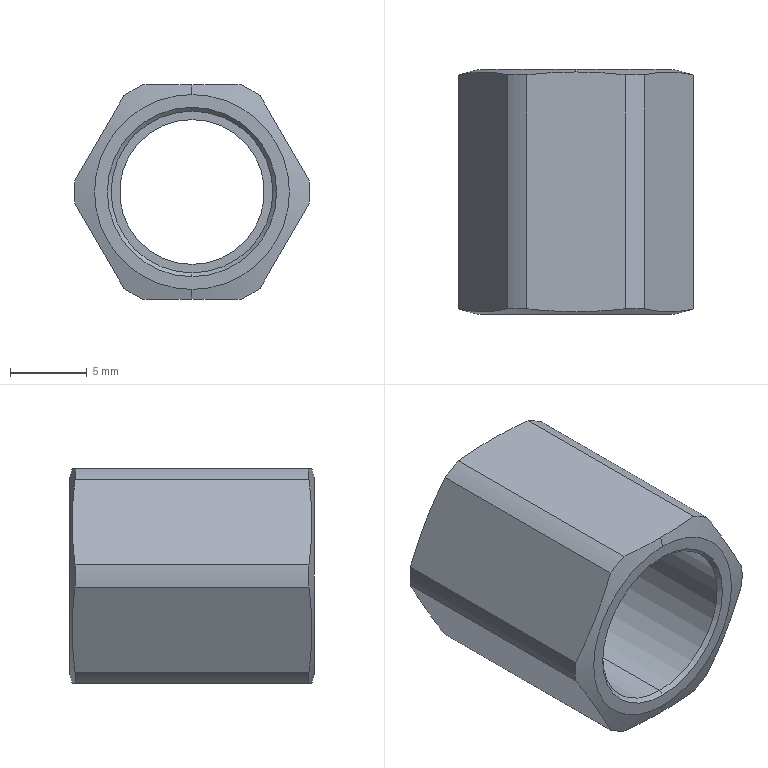Part | STEP file | 11-F-ACA10LM11 | 1 solid | 27 faces | box 15.4 x 16 x 14 mm | volume 1343 mm3 | cylinder 10 | plane 9 | cone 8 | commonest cylinder face diameters 15.4 x6 9.459 x2 10.566 x2
STEP:
#1=CARTESIAN_POINT('',(0.,0.25,-5.283));
#2=VERTEX_POINT('',#1);
#3=CARTESIAN_POINT('',(0.,0.25,5.283));
#4=VERTEX_POINT('',#3);
#5=CARTESIAN_POINT('',(0.,0.25,0.));
#6=DIRECTION('',(0.,1.,0.));
#7=DIRECTION('',(0.,0.,1.));
#8=AXIS2_PLACEMENT_3D('',#5,#6,#7);
#9=CIRCLE('',#8,5.283);
#10=EDGE_CURVE('',#2,#4,#9,.T.);
#11=ORIENTED_EDGE('',*,*,#10,.F.);
#12=CARTESIAN_POINT('',(0.,12.,-5.283));
#13=VERTEX_POINT('',#12);
#14=CARTESIAN_POINT('',(0.,0.,-5.283));
#15=DIRECTION('',(0.,1.,0.));
#16=VECTOR('',#15,1000.);
#17=LINE('',#14,#16);
#18=EDGE_CURVE('',#2,#13,#17,.T.);
#19=ORIENTED_EDGE('',*,*,#18,.T.);
#20=CARTESIAN_POINT('',(0.,12.,5.283));
#21=VERTEX_POINT('',#20);
#22=CARTESIAN_POINT('',(0.,12.,0.));
#23=DIRECTION('',(0.,-1.,0.));
#24=DIRECTION('',(0.,0.,1.));
#25=AXIS2_PLACEMENT_3D('',#22,#23,#24);
#26=CIRCLE('',#25,5.283);
#27=EDGE_CURVE('',#21,#13,#26,.T.);
#28=ORIENTED_EDGE('',*,*,#27,.F.);
#29=CARTESIAN_POINT('',(0.,0.,5.283));
#30=DIRECTION('',(0.,1.,0.));
#31=VECTOR('',#30,1000.);
#32=LINE('',#29,#31);
#33=EDGE_CURVE('',#4,#21,#32,.T.);
#34=ORIENTED_EDGE('',*,*,#33,.F.);
#35=EDGE_LOOP('',(#11,#19,#28,#34));
#36=FACE_OUTER_BOUND('',#35,.T.);
#37=CARTESIAN_POINT('',(0.,0.,0.));
#38=DIRECTION('',(0.,1.,0.));
#39=DIRECTION('',(0.,0.,1.));
#40=AXIS2_PLACEMENT_3D('',#37,#38,#39);
#41=CYLINDRICAL_SURFACE('',#40,5.283);
#42=ADVANCED_FACE('',(#36),#41,.F.);
#43=ORIENTED_EDGE('',*,*,#10,.T.);
#44=CARTESIAN_POINT('',(0.,0.,5.533));
#45=VERTEX_POINT('',#44);
#46=CARTESIAN_POINT('',(0.,0.,5.533));
#47=DIRECTION('',(0.,-0.7071,0.7071));
#48=VECTOR('',#47,1000.);
#49=LINE('',#46,#48);
#50=EDGE_CURVE('',#4,#45,#49,.T.);
#51=ORIENTED_EDGE('',*,*,#50,.T.);
#52=CARTESIAN_POINT('',(0.,0.,-5.533));
#53=VERTEX_POINT('',#52);
#54=CARTESIAN_POINT('',(0.,0.,0.));
#55=DIRECTION('',(0.,1.,0.));
#56=DIRECTION('',(0.,0.,-1.));
#57=AXIS2_PLACEMENT_3D('',#54,#55,#56);
#58=CIRCLE('',#57,5.533);
#59=EDGE_CURVE('',#53,#45,#58,.T.);
#60=ORIENTED_EDGE('',*,*,#59,.F.);
#61=CARTESIAN_POINT('',(0.,0.,-5.533));
#62=DIRECTION('',(0.,-0.7071,-0.7071));
#63=VECTOR('',#62,1000.);
#64=LINE('',#61,#63);
#65=EDGE_CURVE('',#2,#53,#64,.T.);
#66=ORIENTED_EDGE('',*,*,#65,.F.);
#67=EDGE_LOOP('',(#43,#51,#60,#66));
#68=FACE_OUTER_BOUND('',#67,.T.);
#69=CARTESIAN_POINT('',(0.,0.,0.));
#70=DIRECTION('',(0.,-1.,0.));
#71=DIRECTION('',(0.,0.,-1.));
#72=AXIS2_PLACEMENT_3D('',#69,#70,#71);
#73=CONICAL_SURFACE('',#72,5.533,0.7854);
#74=ADVANCED_FACE('',(#68),#73,.F.);
#75=CARTESIAN_POINT('',(0.,12.,-4.729));
#76=VERTEX_POINT('',#75);
#77=CARTESIAN_POINT('',(0.,12.,4.729));
#78=VERTEX_POINT('',#77);
#79=CARTESIAN_POINT('',(0.,12.,0.));
#80=DIRECTION('',(0.,1.,0.));
#81=DIRECTION('',(0.,0.,1.));
#82=AXIS2_PLACEMENT_3D('',#79,#80,#81);
#83=CIRCLE('',#82,4.729);
#84=EDGE_CURVE('',#76,#78,#83,.T.);
#85=ORIENTED_EDGE('',*,*,#84,.F.);
#86=CARTESIAN_POINT('',(0.,15.729,-4.729));
#87=VERTEX_POINT('',#86);
#88=CARTESIAN_POINT('',(0.,0.,-4.729));
#89=DIRECTION('',(0.,1.,0.));
#90=VECTOR('',#89,1000.);
#91=LINE('',#88,#90);
#92=EDGE_CURVE('',#76,#87,#91,.T.);
#93=ORIENTED_EDGE('',*,*,#92,.T.);
#94=CARTESIAN_POINT('',(0.,15.729,4.729));
#95=VERTEX_POINT('',#94);
#96=CARTESIAN_POINT('',(0.,15.729,0.));
#97=DIRECTION('',(0.,-1.,0.));
#98=DIRECTION('',(0.,0.,1.));
#99=AXIS2_PLACEMENT_3D('',#96,#97,#98);
#100=CIRCLE('',#99,4.729);
#101=EDGE_CURVE('',#95,#87,#100,.T.);
#102=ORIENTED_EDGE('',*,*,#101,.F.);
#103=CARTESIAN_POINT('',(0.,0.,4.729));
#104=DIRECTION('',(0.,1.,0.));
#105=VECTOR('',#104,1000.);
#106=LINE('',#103,#105);
#107=EDGE_CURVE('',#78,#95,#106,.T.);
#108=ORIENTED_EDGE('',*,*,#107,.F.);
#109=EDGE_LOOP('',(#85,#93,#102,#108));
#110=FACE_OUTER_BOUND('',#109,.T.);
#111=CARTESIAN_POINT('',(0.,0.,0.));
#112=DIRECTION('',(0.,1.,0.));
#113=DIRECTION('',(0.,0.,1.));
#114=AXIS2_PLACEMENT_3D('',#111,#112,#113);
#115=CYLINDRICAL_SURFACE('',#114,4.729);
#116=ADVANCED_FACE('',(#110),#115,.F.);
#117=ORIENTED_EDGE('',*,*,#101,.T.);
#118=CARTESIAN_POINT('',(0.,16.,-5.));
#119=VERTEX_POINT('',#118);
#120=CARTESIAN_POINT('',(0.,16.,-5.));
#121=DIRECTION('',(0.,0.7071,-0.7071));
#122=VECTOR('',#121,1000.);
#123=LINE('',#120,#122);
#124=EDGE_CURVE('',#87,#119,#123,.T.);
#125=ORIENTED_EDGE('',*,*,#124,.T.);
#126=CARTESIAN_POINT('',(0.,16.,5.));
#127=VERTEX_POINT('',#126);
#128=CARTESIAN_POINT('',(0.,16.,0.));
#129=DIRECTION('',(0.,-1.,0.));
#130=DIRECTION('',(0.,0.,1.));
#131=AXIS2_PLACEMENT_3D('',#128,#129,#130);
#132=CIRCLE('',#131,5.);
#133=EDGE_CURVE('',#127,#119,#132,.T.);
#134=ORIENTED_EDGE('',*,*,#133,.F.);
#135=CARTESIAN_POINT('',(0.,16.,5.));
#136=DIRECTION('',(0.,0.7071,0.7071));
#137=VECTOR('',#136,1000.);
#138=LINE('',#135,#137);
#139=EDGE_CURVE('',#95,#127,#138,.T.);
#140=ORIENTED_EDGE('',*,*,#139,.F.);
#141=EDGE_LOOP('',(#117,#125,#134,#140));
#142=FACE_OUTER_BOUND('',#141,.T.);
#143=CARTESIAN_POINT('',(0.,16.,0.));
#144=DIRECTION('',(0.,1.,0.));
#145=DIRECTION('',(0.,0.,1.));
#146=AXIS2_PLACEMENT_3D('',#143,#144,#145);
#147=CONICAL_SURFACE('',#146,5.,0.7854);
#148=ADVANCED_FACE('',(#142),#147,.F.);
#149=CARTESIAN_POINT('',(0.,0.,-6.364));
#150=VERTEX_POINT('',#149);
#151=CARTESIAN_POINT('',(0.,0.,6.364));
#152=VERTEX_POINT('',#151);
#153=CARTESIAN_POINT('',(0.,0.,0.));
#154=DIRECTION('',(0.,-1.,0.));
#155=DIRECTION('',(0.,0.,1.));
#156=AXIS2_PLACEMENT_3D('',#153,#154,#155);
#157=CIRCLE('',#156,6.364);
#158=EDGE_CURVE('',#150,#152,#157,.T.);
#159=ORIENTED_EDGE('',*,*,#158,.F.);
#160=CARTESIAN_POINT('',(0.,0.1705,-7.));
#161=VERTEX_POINT('',#160);
#162=CARTESIAN_POINT('',(0.,0.3581,-7.7));
#163=DIRECTION('',(0.,0.2588,-0.9659));
#164=VECTOR('',#163,1000.);
#165=LINE('',#162,#164);
#166=EDGE_CURVE('',#150,#161,#165,.T.);
#167=ORIENTED_EDGE('',*,*,#166,.T.);
#168=CARTESIAN_POINT('',(3.208,0.3581,-7.));
#169=VERTEX_POINT('',#168);
#170=CARTESIAN_POINT('',(0.,0.1705,-7.));
#171=CARTESIAN_POINT('',(1.069,0.1705,-7.));
#172=CARTESIAN_POINT('',(2.139,0.2387,-7.));
#173=CARTESIAN_POINT('',(3.208,0.3581,-7.));
#174=B_SPLINE_CURVE_WITH_KNOTS('',3,(#170,#171,#172,#173),.UNSPECIFIED.,.F.,.F.,(4,4),(0.003208,0.006416),.UNSPECIFIED.);
#175=EDGE_CURVE('',#161,#169,#174,.T.);
#176=ORIENTED_EDGE('',*,*,#175,.T.);
#177=CARTESIAN_POINT('',(4.458,0.3581,-6.278));
#178=VERTEX_POINT('',#177);
#179=CARTESIAN_POINT('',(0.,0.3581,0.));
#180=DIRECTION('',(0.,1.,0.));
#181=DIRECTION('',(0.,0.,1.));
#182=AXIS2_PLACEMENT_3D('',#179,#180,#181);
#183=CIRCLE('',#182,7.7);
#184=EDGE_CURVE('',#178,#169,#183,.T.);
#185=ORIENTED_EDGE('',*,*,#184,.F.);
#186=CARTESIAN_POINT('',(7.666,0.3581,-0.722));
#187=VERTEX_POINT('',#186);
#188=CARTESIAN_POINT('',(4.458,0.3581,-6.278));
#189=CARTESIAN_POINT('',(4.993,0.2387,-5.352));
#190=CARTESIAN_POINT('',(6.062,0.1023,-3.5));
#191=CARTESIAN_POINT('',(7.131,0.2387,-1.648));
#192=CARTESIAN_POINT('',(7.666,0.3581,-0.722));
#193=B_SPLINE_CURVE_WITH_KNOTS('',3,(#188,#189,#190,#191,#192),.UNSPECIFIED.,.F.,.F.,(4,1,4),(0.,0.003208,0.006416),.UNSPECIFIED.);
#194=EDGE_CURVE('',#178,#187,#193,.T.);
#195=ORIENTED_EDGE('',*,*,#194,.T.);
#196=CARTESIAN_POINT('',(7.666,0.3581,0.722));
#197=VERTEX_POINT('',#196);
#198=CARTESIAN_POINT('',(0.,0.3581,0.));
#199=DIRECTION('',(0.,1.,0.));
#200=DIRECTION('',(0.,0.,1.));
#201=AXIS2_PLACEMENT_3D('',#198,#199,#200);
#202=CIRCLE('',#201,7.7);
#203=EDGE_CURVE('',#197,#187,#202,.T.);
#204=ORIENTED_EDGE('',*,*,#203,.F.);
#205=CARTESIAN_POINT('',(4.458,0.3581,6.278));
#206=VERTEX_POINT('',#205);
#207=CARTESIAN_POINT('',(7.666,0.3581,0.722));
#208=CARTESIAN_POINT('',(7.131,0.2387,1.648));
#209=CARTESIAN_POINT('',(6.062,0.1023,3.5));
#210=CARTESIAN_POINT('',(4.993,0.2387,5.352));
#211=CARTESIAN_POINT('',(4.458,0.3581,6.278));
#212=B_SPLINE_CURVE_WITH_KNOTS('',3,(#207,#208,#209,#210,#211),.UNSPECIFIED.,.F.,.F.,(4,1,4),(0.,0.003208,0.006416),.UNSPECIFIED.);
#213=EDGE_CURVE('',#197,#206,#212,.T.);
#214=ORIENTED_EDGE('',*,*,#213,.T.);
#215=CARTESIAN_POINT('',(3.208,0.3581,7.));
#216=VERTEX_POINT('',#215);
#217=CARTESIAN_POINT('',(0.,0.3581,0.));
#218=DIRECTION('',(0.,1.,0.));
#219=DIRECTION('',(0.,0.,1.));
#220=AXIS2_PLACEMENT_3D('',#217,#218,#219);
#221=CIRCLE('',#220,7.7);
#222=EDGE_CURVE('',#216,#206,#221,.T.);
#223=ORIENTED_EDGE('',*,*,#222,.F.);
#224=CARTESIAN_POINT('',(0.,0.1705,7.));
#225=VERTEX_POINT('',#224);
#226=CARTESIAN_POINT('',(3.208,0.3581,7.));
#227=CARTESIAN_POINT('',(2.139,0.2387,7.));
#228=CARTESIAN_POINT('',(1.069,0.1705,7.));
#229=CARTESIAN_POINT('',(0.,0.1705,7.));
#230=B_SPLINE_CURVE_WITH_KNOTS('',3,(#226,#227,#228,#229),.UNSPECIFIED.,.F.,.F.,(4,4),(0.,0.003208),.UNSPECIFIED.);
#231=EDGE_CURVE('',#216,#225,#230,.T.);
#232=ORIENTED_EDGE('',*,*,#231,.T.);
#233=CARTESIAN_POINT('',(0.,0.3581,7.7));
#234=DIRECTION('',(0.,0.2588,0.9659));
#235=VECTOR('',#234,1000.);
#236=LINE('',#233,#235);
#237=EDGE_CURVE('',#152,#225,#236,.T.);
#238=ORIENTED_EDGE('',*,*,#237,.F.);
#239=EDGE_LOOP('',(#159,#167,#176,#185,#195,#204,#214,#223,#232,#238));
#240=FACE_OUTER_BOUND('',#239,.T.);
#241=CARTESIAN_POINT('',(0.,0.3581,0.));
#242=DIRECTION('',(0.,1.,0.));
#243=DIRECTION('',(0.,0.,1.));
#244=AXIS2_PLACEMENT_3D('',#241,#242,#243);
#245=CONICAL_SURFACE('',#244,7.7,1.309);
#246=ADVANCED_FACE('',(#240),#245,.T.);
#247=CARTESIAN_POINT('',(0.,16.,6.364));
#248=VERTEX_POINT('',#247);
#249=CARTESIAN_POINT('',(0.,16.,-6.364));
#250=VERTEX_POINT('',#249);
#251=CARTESIAN_POINT('',(0.,16.,0.));
#252=DIRECTION('',(0.,1.,0.));
#253=DIRECTION('',(0.,0.,-1.));
#254=AXIS2_PLACEMENT_3D('',#251,#252,#253);
#255=CIRCLE('',#254,6.364);
#256=EDGE_CURVE('',#248,#250,#255,.T.);
#257=ORIENTED_EDGE('',*,*,#256,.F.);
#258=CARTESIAN_POINT('',(0.,15.829,7.));
#259=VERTEX_POINT('',#258);
#260=CARTESIAN_POINT('',(0.,15.642,7.7));
#261=DIRECTION('',(0.,-0.2588,0.9659));
#262=VECTOR('',#261,1000.);
#263=LINE('',#260,#262);
#264=EDGE_CURVE('',#248,#259,#263,.T.);
#265=ORIENTED_EDGE('',*,*,#264,.T.);
#266=CARTESIAN_POINT('',(3.208,15.642,7.));
#267=VERTEX_POINT('',#266);
#268=CARTESIAN_POINT('',(0.,15.829,7.));
#269=CARTESIAN_POINT('',(1.069,15.829,7.));
#270=CARTESIAN_POINT('',(2.139,15.761,7.));
#271=CARTESIAN_POINT('',(3.208,15.642,7.));
#272=B_SPLINE_CURVE_WITH_KNOTS('',3,(#268,#269,#270,#271),.UNSPECIFIED.,.F.,.F.,(4,4),(0.003208,0.006416),.UNSPECIFIED.);
#273=EDGE_CURVE('',#259,#267,#272,.T.);
#274=ORIENTED_EDGE('',*,*,#273,.T.);
#275=CARTESIAN_POINT('',(4.458,15.642,6.278));
#276=VERTEX_POINT('',#275);
#277=CARTESIAN_POINT('',(0.,15.642,0.));
#278=DIRECTION('',(0.,1.,0.));
#279=DIRECTION('',(0.,0.,-1.));
#280=AXIS2_PLACEMENT_3D('',#277,#278,#279);
#281=CIRCLE('',#280,7.7);
#282=EDGE_CURVE('',#267,#276,#281,.T.);
#283=ORIENTED_EDGE('',*,*,#282,.T.);
#284=CARTESIAN_POINT('',(7.666,15.642,0.722));
#285=VERTEX_POINT('',#284);
#286=CARTESIAN_POINT('',(4.458,15.642,6.278));
#287=CARTESIAN_POINT('',(4.993,15.761,5.352));
#288=CARTESIAN_POINT('',(6.062,15.898,3.5));
#289=CARTESIAN_POINT('',(7.131,15.761,1.648));
#290=CARTESIAN_POINT('',(7.666,15.642,0.722));
#291=B_SPLINE_CURVE_WITH_KNOTS('',3,(#286,#287,#288,#289,#290),.UNSPECIFIED.,.F.,.F.,(4,1,4),(0.,0.003208,0.006416),.UNSPECIFIED.);
#292=EDGE_CURVE('',#276,#285,#291,.T.);
#293=ORIENTED_EDGE('',*,*,#292,.T.);
#294=CARTESIAN_POINT('',(7.666,15.642,-0.722));
#295=VERTEX_POINT('',#294);
#296=CARTESIAN_POINT('',(0.,15.642,0.));
#297=DIRECTION('',(0.,1.,0.));
#298=DIRECTION('',(0.,0.,-1.));
#299=AXIS2_PLACEMENT_3D('',#296,#297,#298);
#300=CIRCLE('',#299,7.7);
#301=EDGE_CURVE('',#285,#295,#300,.T.);
#302=ORIENTED_EDGE('',*,*,#301,.T.);
#303=CARTESIAN_POINT('',(4.458,15.642,-6.278));
#304=VERTEX_POINT('',#303);
#305=CARTESIAN_POINT('',(7.666,15.642,-0.722));
#306=CARTESIAN_POINT('',(7.131,15.761,-1.648));
#307=CARTESIAN_POINT('',(6.062,15.898,-3.5));
#308=CARTESIAN_POINT('',(4.993,15.761,-5.352));
#309=CARTESIAN_POINT('',(4.458,15.642,-6.278));
#310=B_SPLINE_CURVE_WITH_KNOTS('',3,(#305,#306,#307,#308,#309),.UNSPECIFIED.,.F.,.F.,(4,1,4),(0.,0.003208,0.006416),.UNSPECIFIED.);
#311=EDGE_CURVE('',#295,#304,#310,.T.);
#312=ORIENTED_EDGE('',*,*,#311,.T.);
#313=CARTESIAN_POINT('',(3.208,15.642,-7.));
#314=VERTEX_POINT('',#313);
#315=CARTESIAN_POINT('',(0.,15.642,0.));
#316=DIRECTION('',(0.,1.,0.));
#317=DIRECTION('',(0.,0.,-1.));
#318=AXIS2_PLACEMENT_3D('',#315,#316,#317);
#319=CIRCLE('',#318,7.7);
#320=EDGE_CURVE('',#304,#314,#319,.T.);
#321=ORIENTED_EDGE('',*,*,#320,.T.);
#322=CARTESIAN_POINT('',(0.,15.829,-7.));
#323=VERTEX_POINT('',#322);
#324=CARTESIAN_POINT('',(3.208,15.642,-7.));
#325=CARTESIAN_POINT('',(2.139,15.761,-7.));
#326=CARTESIAN_POINT('',(1.069,15.829,-7.));
#327=CARTESIAN_POINT('',(0.,15.829,-7.));
#328=B_SPLINE_CURVE_WITH_KNOTS('',3,(#324,#325,#326,#327),.UNSPECIFIED.,.F.,.F.,(4,4),(0.,0.003208),.UNSPECIFIED.);
#329=EDGE_CURVE('',#314,#323,#328,.T.);
#330=ORIENTED_EDGE('',*,*,#329,.T.);
#331=CARTESIAN_POINT('',(0.,15.642,-7.7));
#332=DIRECTION('',(0.,-0.2588,-0.9659));
#333=VECTOR('',#332,1000.);
#334=LINE('',#331,#333);
#335=EDGE_CURVE('',#250,#323,#334,.T.);
#336=ORIENTED_EDGE('',*,*,#335,.F.);
#337=EDGE_LOOP('',(#257,#265,#274,#283,#293,#302,#312,#321,#330,#336));
#338=FACE_OUTER_BOUND('',#337,.T.);
#339=CARTESIAN_POINT('',(0.,15.642,0.));
#340=DIRECTION('',(0.,-1.,0.));
#341=DIRECTION('',(0.,0.,-1.));
#342=AXIS2_PLACEMENT_3D('',#339,#340,#341);
#343=CONICAL_SURFACE('',#342,7.7,1.309);
#344=ADVANCED_FACE('',(#338),#343,.T.);
#345=ORIENTED_EDGE('',*,*,#18,.F.);
#346=CARTESIAN_POINT('',(0.,0.25,0.));
#347=DIRECTION('',(0.,1.,0.));
#348=DIRECTION('',(0.,0.,1.));
#349=AXIS2_PLACEMENT_3D('',#346,#347,#348);
#350=CIRCLE('',#349,5.283);
#351=EDGE_CURVE('',#4,#2,#350,.T.);
#352=ORIENTED_EDGE('',*,*,#351,.F.);
#353=ORIENTED_EDGE('',*,*,#33,.T.);
#354=CARTESIAN_POINT('',(0.,12.,0.));
#355=DIRECTION('',(0.,-1.,0.));
#356=DIRECTION('',(0.,0.,1.));
#357=AXIS2_PLACEMENT_3D('',#354,#355,#356);
#358=CIRCLE('',#357,5.283);
#359=EDGE_CURVE('',#13,#21,#358,.T.);
#360=ORIENTED_EDGE('',*,*,#359,.F.);
#361=EDGE_LOOP('',(#345,#352,#353,#360));
#362=FACE_OUTER_BOUND('',#361,.T.);
#363=CARTESIAN_POINT('',(0.,0.,0.));
#364=DIRECTION('',(0.,1.,0.));
#365=DIRECTION('',(0.,0.,1.));
#366=AXIS2_PLACEMENT_3D('',#363,#364,#365);
#367=CYLINDRICAL_SURFACE('',#366,5.283);
#368=ADVANCED_FACE('',(#362),#367,.F.);
#369=CARTESIAN_POINT('',(0.,12.,0.));
#370=DIRECTION('',(0.,1.,0.));
#371=DIRECTION('',(0.,0.,1.));
#372=AXIS2_PLACEMENT_3D('',#369,#370,#371);
#373=CIRCLE('',#372,4.729);
#374=EDGE_CURVE('',#78,#76,#373,.T.);
#375=ORIENTED_EDGE('',*,*,#374,.T.);
#376=ORIENTED_EDGE('',*,*,#84,.T.);
#377=EDGE_LOOP('',(#375,#376));
#378=FACE_BOUND('',#377,.T.);
#379=ORIENTED_EDGE('',*,*,#27,.T.);
#380=ORIENTED_EDGE('',*,*,#359,.T.);
#381=EDGE_LOOP('',(#379,#380));
#382=FACE_OUTER_BOUND('',#381,.T.);
#383=CARTESIAN_POINT('',(4.729,12.,0.));
#384=DIRECTION('',(0.,-1.,0.));
#385=DIRECTION('',(0.,0.,-1.));
#386=AXIS2_PLACEMENT_3D('',#383,#384,#385);
#387=PLANE('',#386);
#388=ADVANCED_FACE('',(#378,#382),#387,.T.);
#389=ORIENTED_EDGE('',*,*,#50,.F.);
#390=ORIENTED_EDGE('',*,*,#351,.T.);
#391=ORIENTED_EDGE('',*,*,#65,.T.);
#392=CARTESIAN_POINT('',(0.,0.,0.));
#393=DIRECTION('',(0.,1.,0.));
#394=DIRECTION('',(0.,0.,-1.));
#395=AXIS2_PLACEMENT_3D('',#392,#393,#394);
#396=CIRCLE('',#395,5.533);
#397=EDGE_CURVE('',#45,#53,#396,.T.);
#398=ORIENTED_EDGE('',*,*,#397,.F.);
#399=EDGE_LOOP('',(#389,#390,#391,#398));
#400=FACE_OUTER_BOUND('',#399,.T.);
#401=CARTESIAN_POINT('',(0.,0.,0.));
#402=DIRECTION('',(0.,-1.,0.));
#403=DIRECTION('',(0.,0.,-1.));
#404=AXIS2_PLACEMENT_3D('',#401,#402,#403);
#405=CONICAL_SURFACE('',#404,5.533,0.7854);
#406=ADVANCED_FACE('',(#400),#405,.F.);
#407=ORIENTED_EDGE('',*,*,#92,.F.);
#408=ORIENTED_EDGE('',*,*,#374,.F.);
#409=ORIENTED_EDGE('',*,*,#107,.T.);
#410=CARTESIAN_POINT('',(0.,15.729,0.));
#411=DIRECTION('',(0.,-1.,0.));
#412=DIRECTION('',(0.,0.,1.));
#413=AXIS2_PLACEMENT_3D('',#410,#411,#412);
#414=CIRCLE('',#413,4.729);
#415=EDGE_CURVE('',#87,#95,#414,.T.);
#416=ORIENTED_EDGE('',*,*,#415,.F.);
#417=EDGE_LOOP('',(#407,#408,#409,#416));
#418=FACE_OUTER_BOUND('',#417,.T.);
#419=CARTESIAN_POINT('',(0.,0.,0.));
#420=DIRECTION('',(0.,1.,0.));
#421=DIRECTION('',(0.,0.,1.));
#422=AXIS2_PLACEMENT_3D('',#419,#420,#421);
#423=CYLINDRICAL_SURFACE('',#422,4.729);
#424=ADVANCED_FACE('',(#418),#423,.F.);
#425=ORIENTED_EDGE('',*,*,#59,.T.);
#426=ORIENTED_EDGE('',*,*,#397,.T.);
#427=EDGE_LOOP('',(#425,#426));
#428=FACE_BOUND('',#427,.T.);
#429=CARTESIAN_POINT('',(0.,0.,0.));
#430=DIRECTION('',(0.,-1.,0.));
#431=DIRECTION('',(0.,0.,1.));
#432=AXIS2_PLACEMENT_3D('',#429,#430,#431);
#433=CIRCLE('',#432,6.364);
#434=EDGE_CURVE('',#152,#150,#433,.T.);
#435=ORIENTED_EDGE('',*,*,#434,.T.);
#436=ORIENTED_EDGE('',*,*,#158,.T.);
#437=EDGE_LOOP('',(#435,#436));
#438=FACE_OUTER_BOUND('',#437,.T.);
#439=CARTESIAN_POINT('',(5.533,0.,0.));
#440=DIRECTION('',(0.,-1.,0.));
#441=DIRECTION('',(0.,0.,-1.));
#442=AXIS2_PLACEMENT_3D('',#439,#440,#441);
#443=PLANE('',#442);
#444=ADVANCED_FACE('',(#428,#438),#443,.T.);
#445=ORIENTED_EDGE('',*,*,#124,.F.);
#446=ORIENTED_EDGE('',*,*,#415,.T.);
#447=ORIENTED_EDGE('',*,*,#139,.T.);
#448=CARTESIAN_POINT('',(0.,16.,0.));
#449=DIRECTION('',(0.,-1.,0.));
#450=DIRECTION('',(0.,0.,1.));
#451=AXIS2_PLACEMENT_3D('',#448,#449,#450);
#452=CIRCLE('',#451,5.);
#453=EDGE_CURVE('',#119,#127,#452,.T.);
#454=ORIENTED_EDGE('',*,*,#453,.F.);
#455=EDGE_LOOP('',(#445,#446,#447,#454));
#456=FACE_OUTER_BOUND('',#455,.T.);
#457=CARTESIAN_POINT('',(0.,16.,0.));
#458=DIRECTION('',(0.,1.,0.));
#459=DIRECTION('',(0.,0.,1.));
#460=AXIS2_PLACEMENT_3D('',#457,#458,#459);
#461=CONICAL_SURFACE('',#460,5.,0.7854);
#462=ADVANCED_FACE('',(#456),#461,.F.);
#463=ORIENTED_EDGE('',*,*,#166,.F.);
#464=ORIENTED_EDGE('',*,*,#434,.F.);
#465=ORIENTED_EDGE('',*,*,#237,.T.);
#466=CARTESIAN_POINT('',(-3.208,0.3581,7.));
#467=VERTEX_POINT('',#466);
#468=CARTESIAN_POINT('',(0.,0.1705,7.));
#469=CARTESIAN_POINT('',(-1.069,0.1705,7.));
#470=CARTESIAN_POINT('',(-2.139,0.2387,7.));
#471=CARTESIAN_POINT('',(-3.208,0.3581,7.));
#472=B_SPLINE_CURVE_WITH_KNOTS('',3,(#468,#469,#470,#471),.UNSPECIFIED.,.F.,.F.,(4,4),(0.003208,0.006416),.UNSPECIFIED.);
#473=EDGE_CURVE('',#225,#467,#472,.T.);
#474=ORIENTED_EDGE('',*,*,#473,.T.);
#475=CARTESIAN_POINT('',(-4.458,0.3581,6.278));
#476=VERTEX_POINT('',#475);
#477=CARTESIAN_POINT('',(0.,0.3581,0.));
#478=DIRECTION('',(0.,1.,0.));
#479=DIRECTION('',(0.,0.,1.));
#480=AXIS2_PLACEMENT_3D('',#477,#478,#479);
#481=CIRCLE('',#480,7.7);
#482=EDGE_CURVE('',#476,#467,#481,.T.);
#483=ORIENTED_EDGE('',*,*,#482,.F.);
#484=CARTESIAN_POINT('',(-7.666,0.3581,0.722));
#485=VERTEX_POINT('',#484);
#486=CARTESIAN_POINT('',(-4.458,0.3581,6.278));
#487=CARTESIAN_POINT('',(-4.993,0.2387,5.352));
#488=CARTESIAN_POINT('',(-6.062,0.1023,3.5));
#489=CARTESIAN_POINT('',(-7.131,0.2387,1.648));
#490=CARTESIAN_POINT('',(-7.666,0.3581,0.722));
#491=B_SPLINE_CURVE_WITH_KNOTS('',3,(#486,#487,#488,#489,#490),.UNSPECIFIED.,.F.,.F.,(4,1,4),(0.,0.003208,0.006416),.UNSPECIFIED.);
#492=EDGE_CURVE('',#476,#485,#491,.T.);
#493=ORIENTED_EDGE('',*,*,#492,.T.);
#494=CARTESIAN_POINT('',(-7.666,0.3581,-0.722));
#495=VERTEX_POINT('',#494);
#496=CARTESIAN_POINT('',(0.,0.3581,0.));
#497=DIRECTION('',(0.,1.,0.));
#498=DIRECTION('',(0.,0.,1.));
#499=AXIS2_PLACEMENT_3D('',#496,#497,#498);
#500=CIRCLE('',#499,7.7);
#501=EDGE_CURVE('',#495,#485,#500,.T.);
#502=ORIENTED_EDGE('',*,*,#501,.F.);
#503=CARTESIAN_POINT('',(-4.458,0.3581,-6.278));
#504=VERTEX_POINT('',#503);
#505=CARTESIAN_POINT('',(-7.666,0.3581,-0.722));
#506=CARTESIAN_POINT('',(-7.131,0.2387,-1.648));
#507=CARTESIAN_POINT('',(-6.062,0.1023,-3.5));
#508=CARTESIAN_POINT('',(-4.993,0.2387,-5.352));
#509=CARTESIAN_POINT('',(-4.458,0.3581,-6.278));
#510=B_SPLINE_CURVE_WITH_KNOTS('',3,(#505,#506,#507,#508,#509),.UNSPECIFIED.,.F.,.F.,(4,1,4),(0.,0.003208,0.006416),.UNSPECIFIED.);
#511=EDGE_CURVE('',#495,#504,#510,.T.);
#512=ORIENTED_EDGE('',*,*,#511,.T.);
#513=CARTESIAN_POINT('',(-3.208,0.3581,-7.));
#514=VERTEX_POINT('',#513);
#515=CARTESIAN_POINT('',(0.,0.3581,0.));
#516=DIRECTION('',(0.,1.,0.));
#517=DIRECTION('',(0.,0.,1.));
#518=AXIS2_PLACEMENT_3D('',#515,#516,#517);
#519=CIRCLE('',#518,7.7);
#520=EDGE_CURVE('',#514,#504,#519,.T.);
#521=ORIENTED_EDGE('',*,*,#520,.F.);
#522=CARTESIAN_POINT('',(-3.208,0.3581,-7.));
#523=CARTESIAN_POINT('',(-2.139,0.2387,-7.));
#524=CARTESIAN_POINT('',(-1.069,0.1705,-7.));
#525=CARTESIAN_POINT('',(0.,0.1705,-7.));
#526=B_SPLINE_CURVE_WITH_KNOTS('',3,(#522,#523,#524,#525),.UNSPECIFIED.,.F.,.F.,(4,4),(0.,0.003208),.UNSPECIFIED.);
#527=EDGE_CURVE('',#514,#161,#526,.T.);
#528=ORIENTED_EDGE('',*,*,#527,.T.);
#529=EDGE_LOOP('',(#463,#464,#465,#474,#483,#493,#502,#512,#521,#528));
#530=FACE_OUTER_BOUND('',#529,.T.);
#531=CARTESIAN_POINT('',(0.,0.3581,0.));
#532=DIRECTION('',(0.,1.,0.));
#533=DIRECTION('',(0.,0.,1.));
#534=AXIS2_PLACEMENT_3D('',#531,#532,#533);
#535=CONICAL_SURFACE('',#534,7.7,1.309);
#536=ADVANCED_FACE('',(#530),#535,.T.);
#537=CARTESIAN_POINT('',(0.,16.,0.));
#538=DIRECTION('',(0.,1.,0.));
#539=DIRECTION('',(0.,0.,-1.));
#540=AXIS2_PLACEMENT_3D('',#537,#538,#539);
#541=CIRCLE('',#540,6.364);
#542=EDGE_CURVE('',#250,#248,#541,.T.);
#543=ORIENTED_EDGE('',*,*,#542,.T.);
#544=ORIENTED_EDGE('',*,*,#256,.T.);
#545=EDGE_LOOP('',(#543,#544));
#546=FACE_OUTER_BOUND('',#545,.T.);
#547=ORIENTED_EDGE('',*,*,#133,.T.);
#548=ORIENTED_EDGE('',*,*,#453,.T.);
#549=EDGE_LOOP('',(#547,#548));
#550=FACE_BOUND('',#549,.T.);
#551=CARTESIAN_POINT('',(6.364,16.,0.));
#552=DIRECTION('',(0.,1.,0.));
#553=DIRECTION('',(0.,0.,1.));
#554=AXIS2_PLACEMENT_3D('',#551,#552,#553);
#555=PLANE('',#554);
#556=ADVANCED_FACE('',(#546,#550),#555,.T.);
#557=CARTESIAN_POINT('',(-3.208,15.642,-7.));
#558=VERTEX_POINT('',#557);
#559=CARTESIAN_POINT('',(-3.208,16.,-7.));
#560=DIRECTION('',(0.,-1.,0.));
#561=VECTOR('',#560,1000.);
#562=LINE('',#559,#561);
#563=EDGE_CURVE('',#558,#514,#562,.T.);
#564=ORIENTED_EDGE('',*,*,#563,.F.);
#565=CARTESIAN_POINT('',(0.,15.829,-7.));
#566=CARTESIAN_POINT('',(-1.069,15.829,-7.));
#567=CARTESIAN_POINT('',(-2.139,15.761,-7.));
#568=CARTESIAN_POINT('',(-3.208,15.642,-7.));
#569=B_SPLINE_CURVE_WITH_KNOTS('',3,(#565,#566,#567,#568),.UNSPECIFIED.,.F.,.F.,(4,4),(0.003208,0.006416),.UNSPECIFIED.);
#570=EDGE_CURVE('',#323,#558,#569,.T.);
#571=ORIENTED_EDGE('',*,*,#570,.F.);
#572=ORIENTED_EDGE('',*,*,#329,.F.);
#573=CARTESIAN_POINT('',(3.208,16.,-7.));
#574=DIRECTION('',(0.,1.,0.));
#575=VECTOR('',#574,1000.);
#576=LINE('',#573,#575);
#577=EDGE_CURVE('',#169,#314,#576,.T.);
#578=ORIENTED_EDGE('',*,*,#577,.F.);
#579=ORIENTED_EDGE('',*,*,#175,.F.);
#580=ORIENTED_EDGE('',*,*,#527,.F.);
#581=EDGE_LOOP('',(#564,#571,#572,#578,#579,#580));
#582=FACE_OUTER_BOUND('',#581,.T.);
#583=CARTESIAN_POINT('',(4.041,16.,-7.));
#584=DIRECTION('',(0.,0.,1.));
#585=DIRECTION('',(1.,0.,0.));
#586=AXIS2_PLACEMENT_3D('',#583,#584,#585);
#587=PLANE('',#586);
#588=ADVANCED_FACE('',(#582),#587,.F.);
#589=CARTESIAN_POINT('',(-7.666,15.642,-0.722));
#590=VERTEX_POINT('',#589);
#591=CARTESIAN_POINT('',(-7.666,16.,-0.722));
#592=DIRECTION('',(0.,-1.,0.));
#593=VECTOR('',#592,1000.);
#594=LINE('',#591,#593);
#595=EDGE_CURVE('',#590,#495,#594,.T.);
#596=ORIENTED_EDGE('',*,*,#595,.F.);
#597=CARTESIAN_POINT('',(-4.458,15.642,-6.278));
#598=VERTEX_POINT('',#597);
#599=CARTESIAN_POINT('',(-4.458,15.642,-6.278));
#600=CARTESIAN_POINT('',(-4.993,15.761,-5.352));
#601=CARTESIAN_POINT('',(-6.062,15.898,-3.5));
#602=CARTESIAN_POINT('',(-7.131,15.761,-1.648));
#603=CARTESIAN_POINT('',(-7.666,15.642,-0.722));
#604=B_SPLINE_CURVE_WITH_KNOTS('',3,(#599,#600,#601,#602,#603),.UNSPECIFIED.,.F.,.F.,(4,1,4),(0.,0.003208,0.006416),.UNSPECIFIED.);
#605=EDGE_CURVE('',#598,#590,#604,.T.);
#606=ORIENTED_EDGE('',*,*,#605,.F.);
#607=CARTESIAN_POINT('',(-4.458,16.,-6.278));
#608=DIRECTION('',(0.,1.,0.));
#609=VECTOR('',#608,1000.);
#610=LINE('',#607,#609);
#611=EDGE_CURVE('',#504,#598,#610,.T.);
#612=ORIENTED_EDGE('',*,*,#611,.F.);
#613=ORIENTED_EDGE('',*,*,#511,.F.);
#614=EDGE_LOOP('',(#596,#606,#612,#613));
#615=FACE_OUTER_BOUND('',#614,.T.);
#616=CARTESIAN_POINT('',(-4.041,16.,-7.));
#617=DIRECTION('',(0.866,0.,0.5));
#618=DIRECTION('',(0.5,0.,-0.866));
#619=AXIS2_PLACEMENT_3D('',#616,#617,#618);
#620=PLANE('',#619);
#621=ADVANCED_FACE('',(#615),#620,.F.);
#622=CARTESIAN_POINT('',(-4.458,15.642,6.278));
#623=VERTEX_POINT('',#622);
#624=CARTESIAN_POINT('',(-4.458,16.,6.278));
#625=DIRECTION('',(0.,-1.,0.));
#626=VECTOR('',#625,1000.);
#627=LINE('',#624,#626);
#628=EDGE_CURVE('',#623,#476,#627,.T.);
#629=ORIENTED_EDGE('',*,*,#628,.F.);
#630=CARTESIAN_POINT('',(-7.666,15.642,0.722));
#631=VERTEX_POINT('',#630);
#632=CARTESIAN_POINT('',(-7.666,15.642,0.722));
#633=CARTESIAN_POINT('',(-7.131,15.761,1.648));
#634=CARTESIAN_POINT('',(-6.062,15.898,3.5));
#635=CARTESIAN_POINT('',(-4.993,15.761,5.352));
#636=CARTESIAN_POINT('',(-4.458,15.642,6.278));
#637=B_SPLINE_CURVE_WITH_KNOTS('',3,(#632,#633,#634,#635,#636),.UNSPECIFIED.,.F.,.F.,(4,1,4),(0.,0.003208,0.006416),.UNSPECIFIED.);
#638=EDGE_CURVE('',#631,#623,#637,.T.);
#639=ORIENTED_EDGE('',*,*,#638,.F.);
#640=CARTESIAN_POINT('',(-7.666,16.,0.722));
#641=DIRECTION('',(0.,1.,0.));
#642=VECTOR('',#641,1000.);
#643=LINE('',#640,#642);
#644=EDGE_CURVE('',#485,#631,#643,.T.);
#645=ORIENTED_EDGE('',*,*,#644,.F.);
#646=ORIENTED_EDGE('',*,*,#492,.F.);
#647=EDGE_LOOP('',(#629,#639,#645,#646));
#648=FACE_OUTER_BOUND('',#647,.T.);
#649=CARTESIAN_POINT('',(-8.083,16.,0.));
#650=DIRECTION('',(0.866,0.,-0.5));
#651=DIRECTION('',(-0.5,0.,-0.866));
#652=AXIS2_PLACEMENT_3D('',#649,#650,#651);
#653=PLANE('',#652);
#654=ADVANCED_FACE('',(#648),#653,.F.);
#655=CARTESIAN_POINT('',(3.208,16.,7.));
#656=DIRECTION('',(0.,-1.,0.));
#657=VECTOR('',#656,1000.);
#658=LINE('',#655,#657);
#659=EDGE_CURVE('',#267,#216,#658,.T.);
#660=ORIENTED_EDGE('',*,*,#659,.F.);
#661=ORIENTED_EDGE('',*,*,#273,.F.);
#662=CARTESIAN_POINT('',(-3.208,15.642,7.));
#663=VERTEX_POINT('',#662);
#664=CARTESIAN_POINT('',(-3.208,15.642,7.));
#665=CARTESIAN_POINT('',(-2.139,15.761,7.));
#666=CARTESIAN_POINT('',(-1.069,15.829,7.));
#667=CARTESIAN_POINT('',(0.,15.829,7.));
#668=B_SPLINE_CURVE_WITH_KNOTS('',3,(#664,#665,#666,#667),.UNSPECIFIED.,.F.,.F.,(4,4),(0.,0.003208),.UNSPECIFIED.);
#669=EDGE_CURVE('',#663,#259,#668,.T.);
#670=ORIENTED_EDGE('',*,*,#669,.F.);
#671=CARTESIAN_POINT('',(-3.208,16.,7.));
#672=DIRECTION('',(0.,1.,0.));
#673=VECTOR('',#672,1000.);
#674=LINE('',#671,#673);
#675=EDGE_CURVE('',#467,#663,#674,.T.);
#676=ORIENTED_EDGE('',*,*,#675,.F.);
#677=ORIENTED_EDGE('',*,*,#473,.F.);
#678=ORIENTED_EDGE('',*,*,#231,.F.);
#679=EDGE_LOOP('',(#660,#661,#670,#676,#677,#678));
#680=FACE_OUTER_BOUND('',#679,.T.);
#681=CARTESIAN_POINT('',(-4.041,16.,7.));
#682=DIRECTION('',(0.,0.,-1.));
#683=DIRECTION('',(-1.,0.,0.));
#684=AXIS2_PLACEMENT_3D('',#681,#682,#683);
#685=PLANE('',#684);
#686=ADVANCED_FACE('',(#680),#685,.F.);
#687=CARTESIAN_POINT('',(7.666,16.,0.722));
#688=DIRECTION('',(0.,-1.,0.));
#689=VECTOR('',#688,1000.);
#690=LINE('',#687,#689);
#691=EDGE_CURVE('',#285,#197,#690,.T.);
#692=ORIENTED_EDGE('',*,*,#691,.F.);
#693=ORIENTED_EDGE('',*,*,#292,.F.);
#694=CARTESIAN_POINT('',(4.458,16.,6.278));
#695=DIRECTION('',(0.,1.,0.));
#696=VECTOR('',#695,1000.);
#697=LINE('',#694,#696);
#698=EDGE_CURVE('',#206,#276,#697,.T.);
#699=ORIENTED_EDGE('',*,*,#698,.F.);
#700=ORIENTED_EDGE('',*,*,#213,.F.);
#701=EDGE_LOOP('',(#692,#693,#699,#700));
#702=FACE_OUTER_BOUND('',#701,.T.);
#703=CARTESIAN_POINT('',(4.041,16.,7.));
#704=DIRECTION('',(-0.866,0.,-0.5));
#705=DIRECTION('',(-0.5,0.,0.866));
#706=AXIS2_PLACEMENT_3D('',#703,#704,#705);
#707=PLANE('',#706);
#708=ADVANCED_FACE('',(#702),#707,.F.);
#709=CARTESIAN_POINT('',(4.458,16.,-6.278));
#710=DIRECTION('',(0.,-1.,0.));
#711=VECTOR('',#710,1000.);
#712=LINE('',#709,#711);
#713=EDGE_CURVE('',#304,#178,#712,.T.);
#714=ORIENTED_EDGE('',*,*,#713,.F.);
#715=ORIENTED_EDGE('',*,*,#311,.F.);
#716=CARTESIAN_POINT('',(7.666,16.,-0.722));
#717=DIRECTION('',(0.,1.,0.));
#718=VECTOR('',#717,1000.);
#719=LINE('',#716,#718);
#720=EDGE_CURVE('',#187,#295,#719,.T.);
#721=ORIENTED_EDGE('',*,*,#720,.F.);
#722=ORIENTED_EDGE('',*,*,#194,.F.);
#723=EDGE_LOOP('',(#714,#715,#721,#722));
#724=FACE_OUTER_BOUND('',#723,.T.);
#725=CARTESIAN_POINT('',(8.083,16.,0.));
#726=DIRECTION('',(-0.866,0.,0.5));
#727=DIRECTION('',(0.5,0.,0.866));
#728=AXIS2_PLACEMENT_3D('',#725,#726,#727);
#729=PLANE('',#728);
#730=ADVANCED_FACE('',(#724),#729,.F.);
#731=ORIENTED_EDGE('',*,*,#264,.F.);
#732=ORIENTED_EDGE('',*,*,#542,.F.);
#733=ORIENTED_EDGE('',*,*,#335,.T.);
#734=ORIENTED_EDGE('',*,*,#570,.T.);
#735=CARTESIAN_POINT('',(0.,15.642,0.));
#736=DIRECTION('',(0.,1.,0.));
#737=DIRECTION('',(0.,0.,-1.));
#738=AXIS2_PLACEMENT_3D('',#735,#736,#737);
#739=CIRCLE('',#738,7.7);
#740=EDGE_CURVE('',#558,#598,#739,.T.);
#741=ORIENTED_EDGE('',*,*,#740,.T.);
#742=ORIENTED_EDGE('',*,*,#605,.T.);
#743=CARTESIAN_POINT('',(0.,15.642,0.));
#744=DIRECTION('',(0.,1.,0.));
#745=DIRECTION('',(0.,0.,-1.));
#746=AXIS2_PLACEMENT_3D('',#743,#744,#745);
#747=CIRCLE('',#746,7.7);
#748=EDGE_CURVE('',#590,#631,#747,.T.);
#749=ORIENTED_EDGE('',*,*,#748,.T.);
#750=ORIENTED_EDGE('',*,*,#638,.T.);
#751=CARTESIAN_POINT('',(0.,15.642,0.));
#752=DIRECTION('',(0.,1.,0.));
#753=DIRECTION('',(0.,0.,-1.));
#754=AXIS2_PLACEMENT_3D('',#751,#752,#753);
#755=CIRCLE('',#754,7.7);
#756=EDGE_CURVE('',#623,#663,#755,.T.);
#757=ORIENTED_EDGE('',*,*,#756,.T.);
#758=ORIENTED_EDGE('',*,*,#669,.T.);
#759=EDGE_LOOP('',(#731,#732,#733,#734,#741,#742,#749,#750,#757,#758));
#760=FACE_OUTER_BOUND('',#759,.T.);
#761=CARTESIAN_POINT('',(0.,15.642,0.));
#762=DIRECTION('',(0.,-1.,0.));
#763=DIRECTION('',(0.,0.,-1.));
#764=AXIS2_PLACEMENT_3D('',#761,#762,#763);
#765=CONICAL_SURFACE('',#764,7.7,1.309);
#766=ADVANCED_FACE('',(#760),#765,.T.);
#767=ORIENTED_EDGE('',*,*,#520,.T.);
#768=ORIENTED_EDGE('',*,*,#611,.T.);
#769=ORIENTED_EDGE('',*,*,#740,.F.);
#770=ORIENTED_EDGE('',*,*,#563,.T.);
#771=EDGE_LOOP('',(#767,#768,#769,#770));
#772=FACE_OUTER_BOUND('',#771,.T.);
#773=CARTESIAN_POINT('',(0.,16.,0.));
#774=DIRECTION('',(0.,1.,0.));
#775=DIRECTION('',(0.,0.,1.));
#776=AXIS2_PLACEMENT_3D('',#773,#774,#775);
#777=CYLINDRICAL_SURFACE('',#776,7.7);
#778=ADVANCED_FACE('',(#772),#777,.T.);
#779=ORIENTED_EDGE('',*,*,#184,.T.);
#780=ORIENTED_EDGE('',*,*,#577,.T.);
#781=ORIENTED_EDGE('',*,*,#320,.F.);
#782=ORIENTED_EDGE('',*,*,#713,.T.);
#783=EDGE_LOOP('',(#779,#780,#781,#782));
#784=FACE_OUTER_BOUND('',#783,.T.);
#785=CARTESIAN_POINT('',(0.,16.,0.));
#786=DIRECTION('',(0.,1.,0.));
#787=DIRECTION('',(0.,0.,1.));
#788=AXIS2_PLACEMENT_3D('',#785,#786,#787);
#789=CYLINDRICAL_SURFACE('',#788,7.7);
#790=ADVANCED_FACE('',(#784),#789,.T.);
#791=ORIENTED_EDGE('',*,*,#748,.F.);
#792=ORIENTED_EDGE('',*,*,#595,.T.);
#793=ORIENTED_EDGE('',*,*,#501,.T.);
#794=ORIENTED_EDGE('',*,*,#644,.T.);
#795=EDGE_LOOP('',(#791,#792,#793,#794));
#796=FACE_OUTER_BOUND('',#795,.T.);
#797=CARTESIAN_POINT('',(0.,16.,0.));
#798=DIRECTION('',(0.,1.,0.));
#799=DIRECTION('',(0.,0.,1.));
#800=AXIS2_PLACEMENT_3D('',#797,#798,#799);
#801=CYLINDRICAL_SURFACE('',#800,7.7);
#802=ADVANCED_FACE('',(#796),#801,.T.);
#803=ORIENTED_EDGE('',*,*,#482,.T.);
#804=ORIENTED_EDGE('',*,*,#675,.T.);
#805=ORIENTED_EDGE('',*,*,#756,.F.);
#806=ORIENTED_EDGE('',*,*,#628,.T.);
#807=EDGE_LOOP('',(#803,#804,#805,#806));
#808=FACE_OUTER_BOUND('',#807,.T.);
#809=CARTESIAN_POINT('',(0.,16.,0.));
#810=DIRECTION('',(0.,1.,0.));
#811=DIRECTION('',(0.,0.,1.));
#812=AXIS2_PLACEMENT_3D('',#809,#810,#811);
#813=CYLINDRICAL_SURFACE('',#812,7.7);
#814=ADVANCED_FACE('',(#808),#813,.T.);
#815=ORIENTED_EDGE('',*,*,#222,.T.);
#816=ORIENTED_EDGE('',*,*,#698,.T.);
#817=ORIENTED_EDGE('',*,*,#282,.F.);
#818=ORIENTED_EDGE('',*,*,#659,.T.);
#819=EDGE_LOOP('',(#815,#816,#817,#818));
#820=FACE_OUTER_BOUND('',#819,.T.);
#821=CARTESIAN_POINT('',(0.,16.,0.));
#822=DIRECTION('',(0.,1.,0.));
#823=DIRECTION('',(0.,0.,1.));
#824=AXIS2_PLACEMENT_3D('',#821,#822,#823);
#825=CYLINDRICAL_SURFACE('',#824,7.7);
#826=ADVANCED_FACE('',(#820),#825,.T.);
#827=ORIENTED_EDGE('',*,*,#301,.F.);
#828=ORIENTED_EDGE('',*,*,#691,.T.);
#829=ORIENTED_EDGE('',*,*,#203,.T.);
#830=ORIENTED_EDGE('',*,*,#720,.T.);
#831=EDGE_LOOP('',(#827,#828,#829,#830));
#832=FACE_OUTER_BOUND('',#831,.T.);
#833=CARTESIAN_POINT('',(0.,16.,0.));
#834=DIRECTION('',(0.,1.,0.));
#835=DIRECTION('',(0.,0.,1.));
#836=AXIS2_PLACEMENT_3D('',#833,#834,#835);
#837=CYLINDRICAL_SURFACE('',#836,7.7);
#838=ADVANCED_FACE('',(#832),#837,.T.);
#839=CLOSED_SHELL('',(#42,#74,#116,#148,#246,#344,#368,#388,#406,#424,#444,#462,#536,#556,#588,#621,#654,#686,#708,#730,#766,#778,#790,#802,#814,#826,#838));
#840=MANIFOLD_SOLID_BREP('',#839);
#841=CARTESIAN_POINT('',(0.,0.,0.));
#842=DIRECTION('',(0.,0.,1.));
#843=DIRECTION('',(1.,0.,0.));
#844=AXIS2_PLACEMENT_3D('',#841,#842,#843);
#845=(LENGTH_UNIT()NAMED_UNIT(*)SI_UNIT(.MILLI.,.METRE.));
#846=UNCERTAINTY_MEASURE_WITH_UNIT(LENGTH_MEASURE(0.00001),#845,'','');
#847=(NAMED_UNIT(*)PLANE_ANGLE_UNIT()SI_UNIT($,.RADIAN.));
#848=(NAMED_UNIT(*)SI_UNIT($,.STERADIAN.)SOLID_ANGLE_UNIT());
#849=(GEOMETRIC_REPRESENTATION_CONTEXT(3)GLOBAL_UNCERTAINTY_ASSIGNED_CONTEXT((#846))GLOBAL_UNIT_ASSIGNED_CONTEXT((#845,#847,#848))REPRESENTATION_CONTEXT('',''));
#850=ADVANCED_BREP_SHAPE_REPRESENTATION('',(#840,#844),#849);